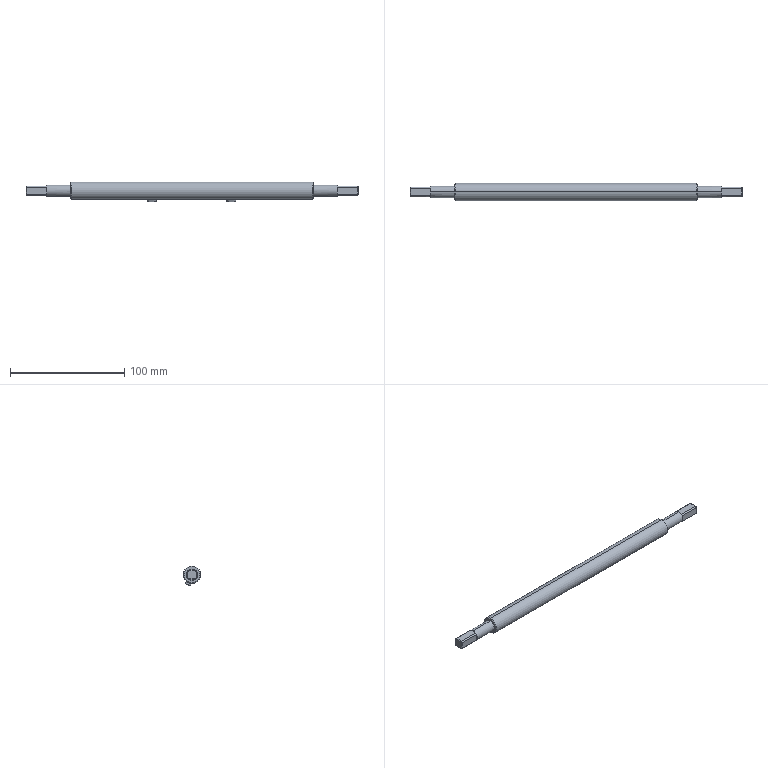Part | SolidWorks | features ICE 3, Chamfer 1, Cut 1, Extrusion 1, Fillet 1, MirrorPattern 1 | 3 solids | 72 faces | box 290 x 15 x 17.22 mm | volume 43129 mm3 | plane 42 | cylinder 18 | cone 12 | commonest cylinder face diameters 5 x12 10 x4 15 x2